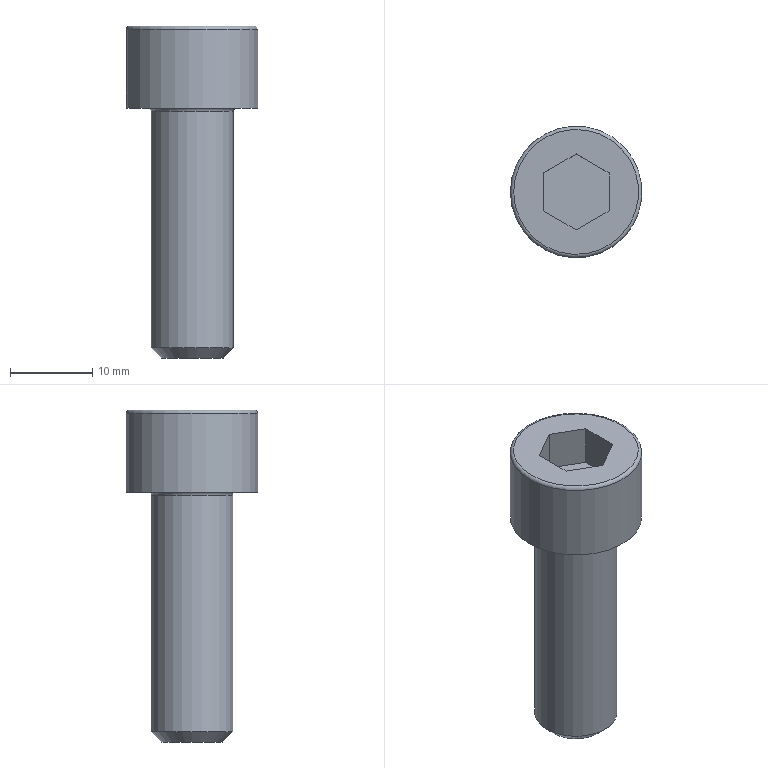Part | STEP file | solid 157 | 1 solid | 15 faces | box 16 x 16 x 40.4 mm | volume 4098 mm3 | plane 10 | cylinder 2 | torus 2 | cone 1 | commonest cylinder face diameters 10 x1 16 x1